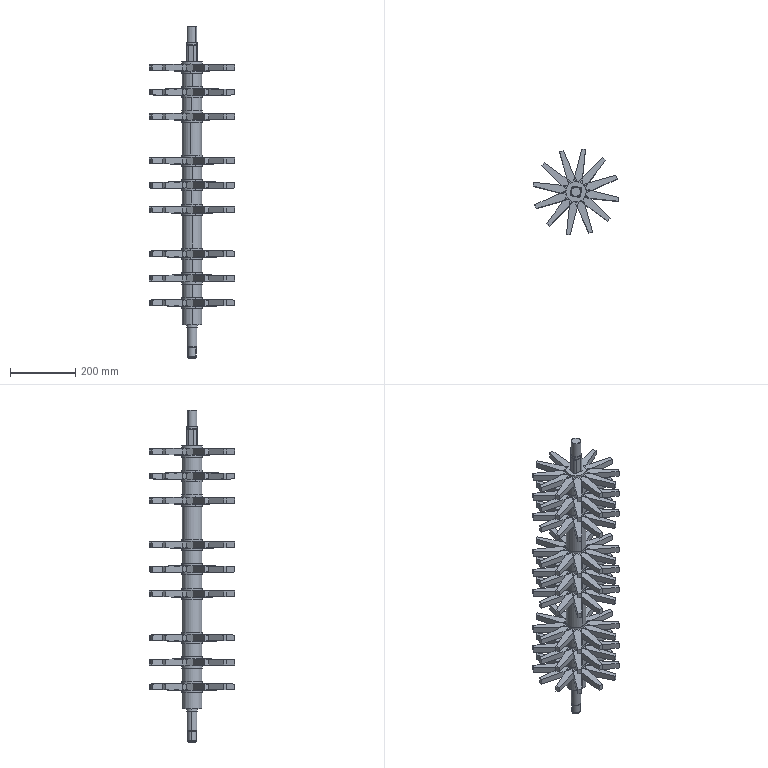Part | SolidWorks | features LayoutProfileFeature 1 | 26 solids | 1684 faces | box 262.006 x 262.006 x 1016 mm | volume 5789700 mm3 | plane 1524 | cylinder 124 | cone 32 | spline 4 | commonest cylinder face diameters 62 x36 15 x20 40 x18 60 x18 9 x12 24 x4